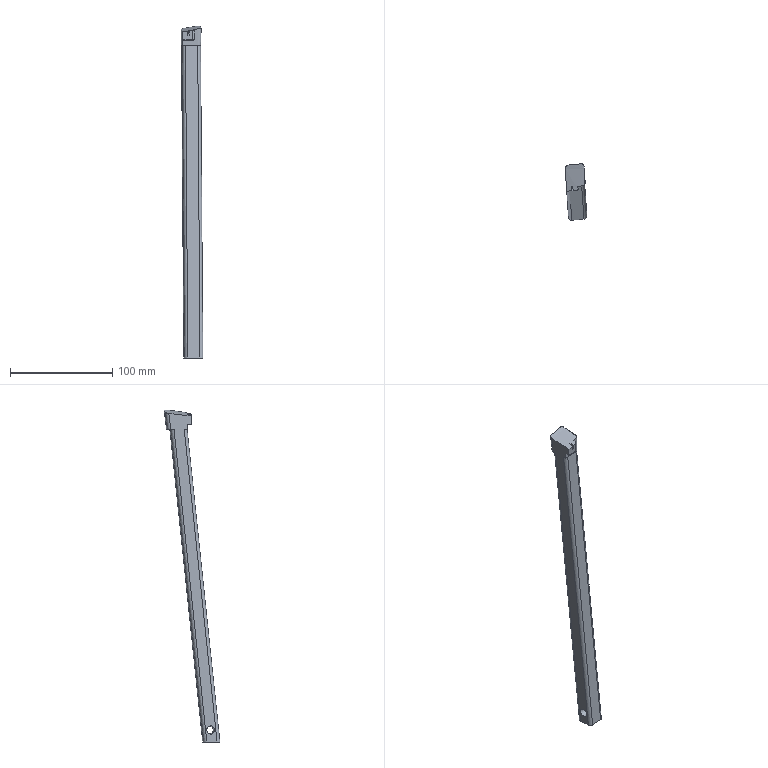Part | STEP file | 车灯-后视镜_id534_x_t | 1 solid | 31 faces | box 21.278 x 54.656 x 325.478 mm | volume 91960 mm3 | plane 17 | cylinder 9 | spline 5 | commonest cylinder face diameters 6 x7 1.018 x1 8 x1